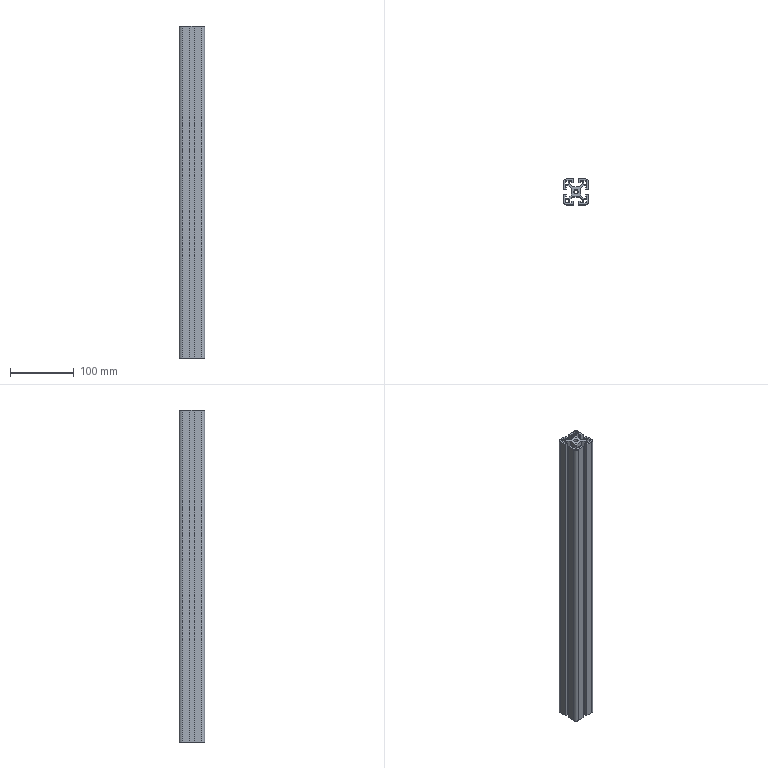Part | STEP file | 4040-520 | 1 solid | 88 faces | box 40 x 40 x 520 mm | volume 366052 mm3 | plane 78 | cylinder 10 | commonest cylinder face diameters 4 x4 10 x4 6.8 x2